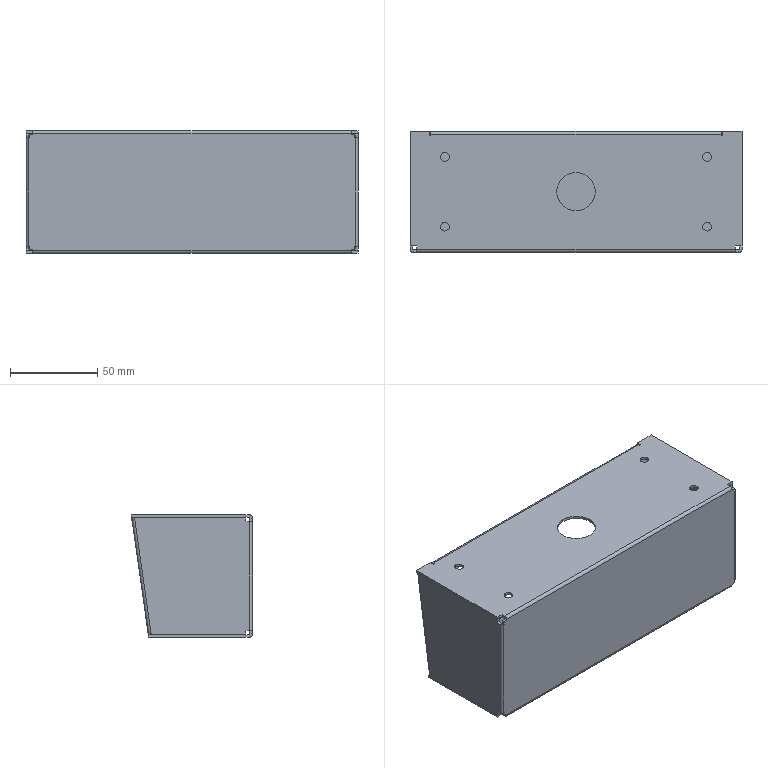Part | STEP file | Control Box Housing | 1 solid | 110 faces | box 190 x 69.286 x 70 mm | volume 74278 mm3 | plane 76 | cylinder 34 | commonest cylinder face diameters 3.2 x16 0.2 x8 5 x8 22 x2